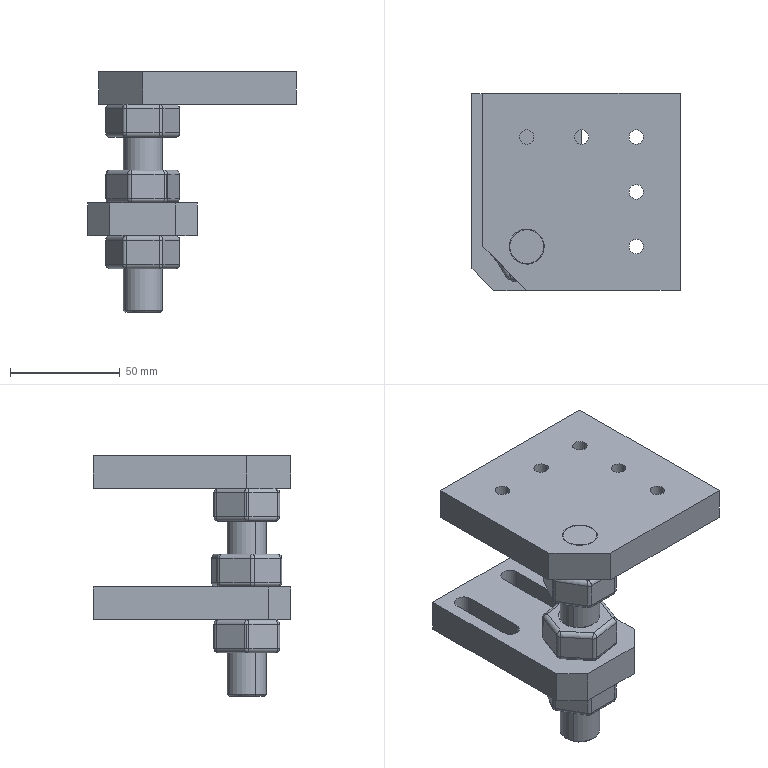Part | SolidWorks | 6 solids | 231 faces | box 95 x 90 x 110 mm | volume 212386 mm3 | cylinder 135 | plane 53 | sphere 36 | cone 4 | spline 3 | commonest cylinder face diameters 4 x57 18 x50 6.6 x10 12 x10 8.4 x4 15.5 x2